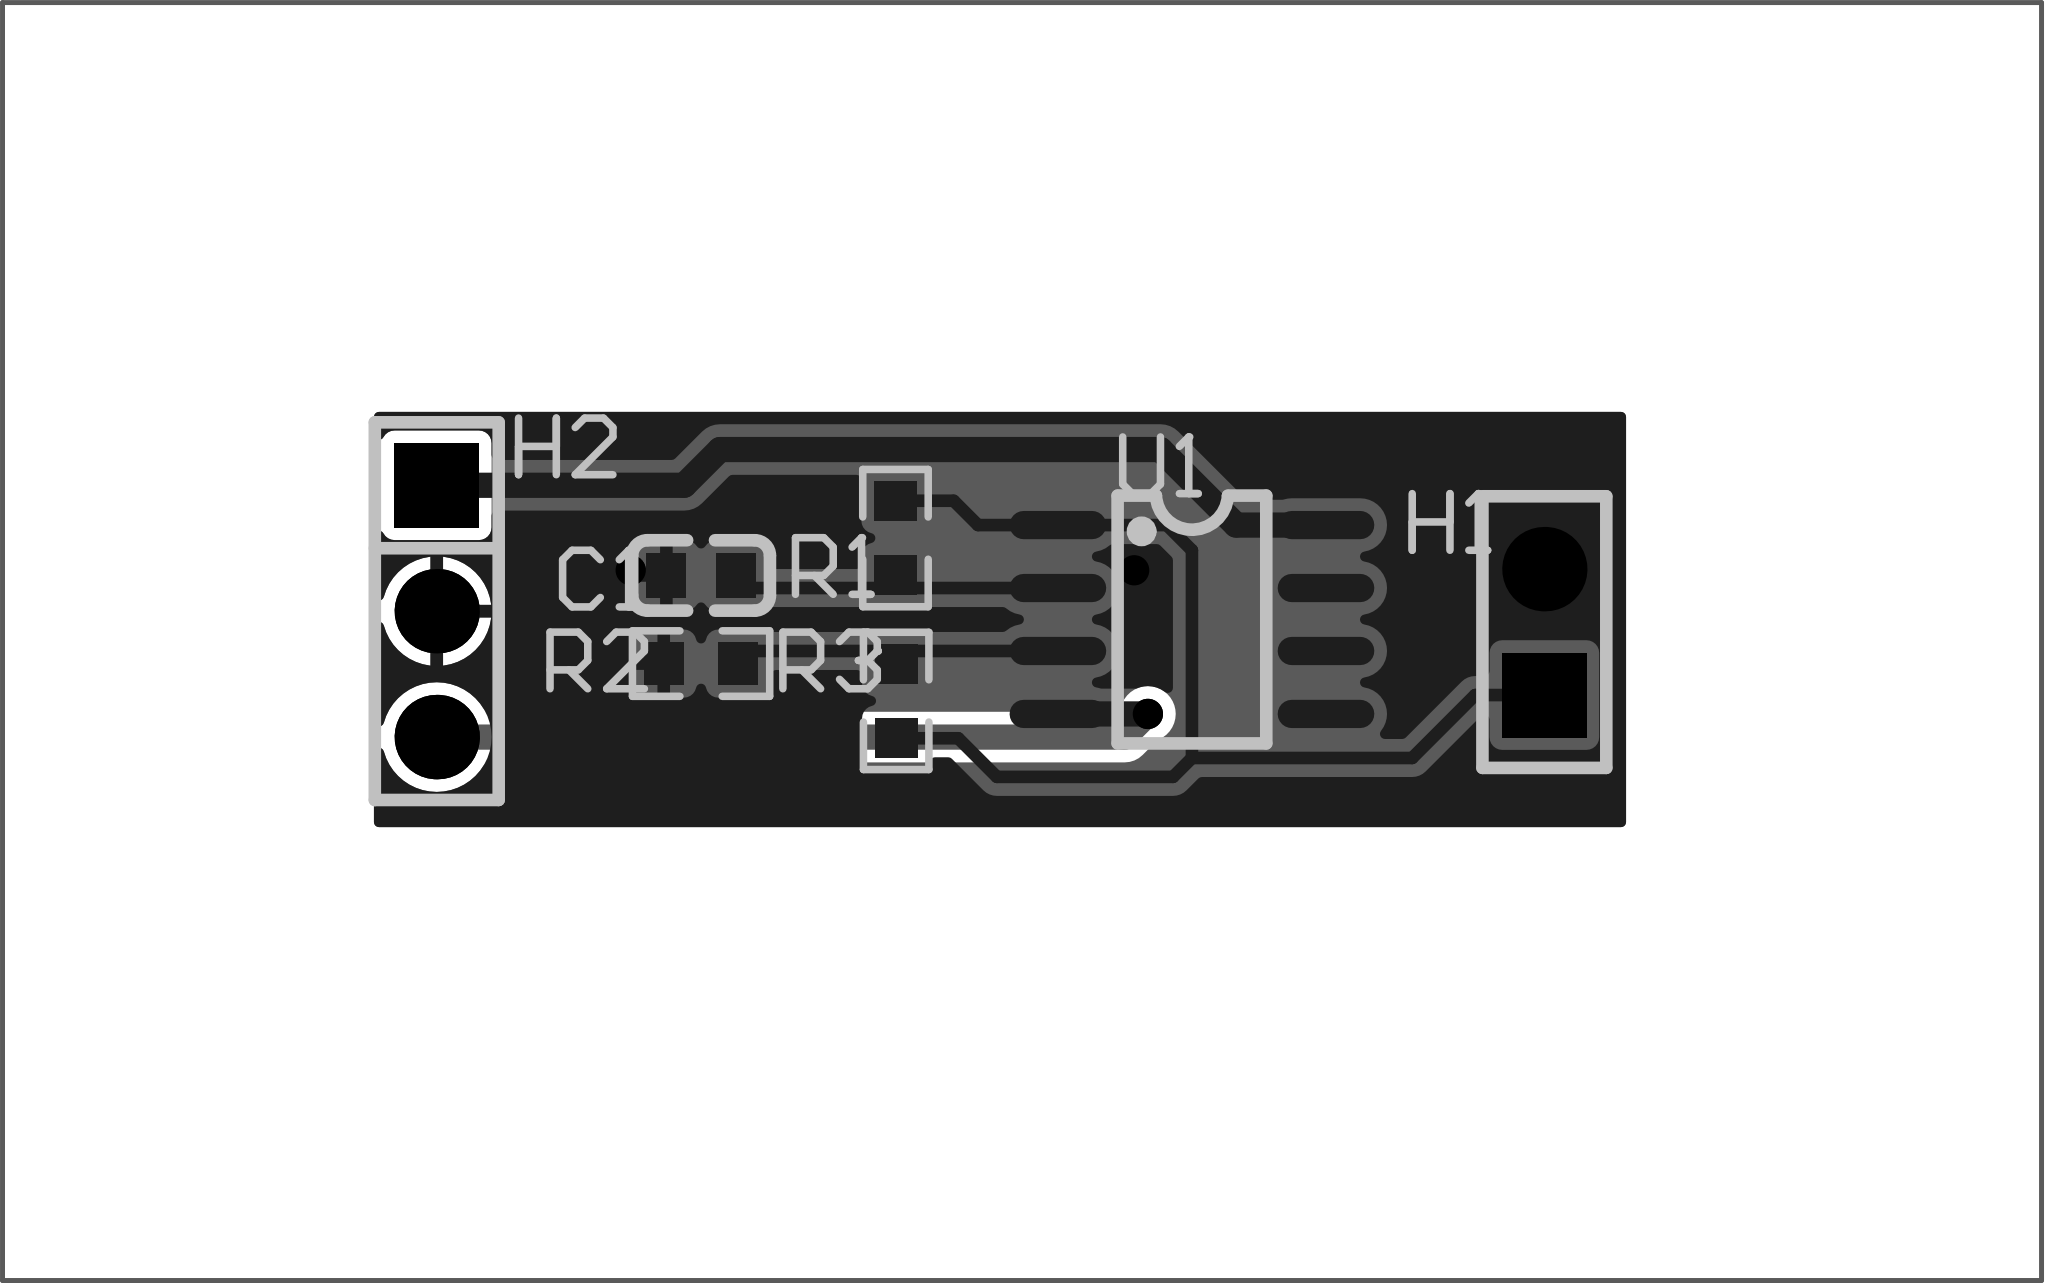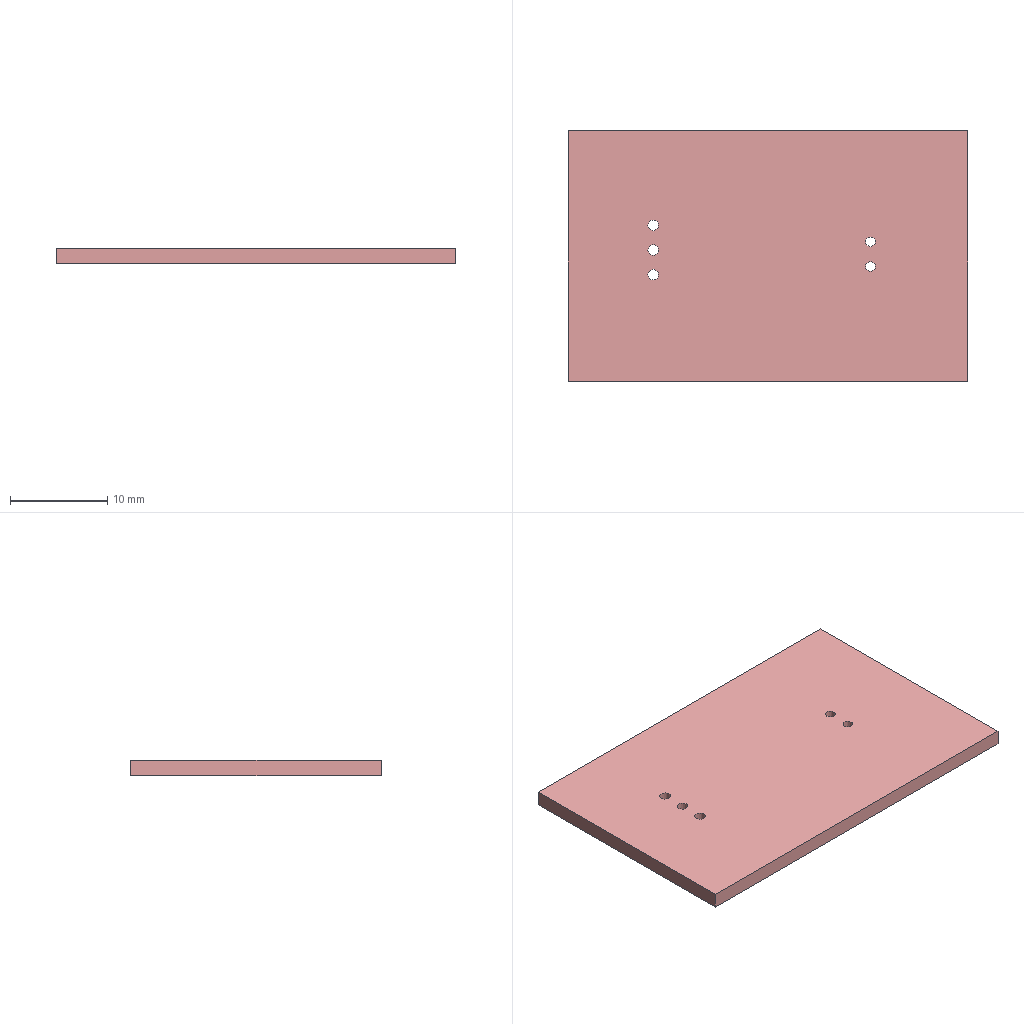Circuit board layout | Altium Designer | box 41.1 x 25.8 x 1.6 mm
Layer stack:
# Altium Designer layer stack of  (unit mm; dielectric type: 0 none, 1 core, 2 prepreg, 3 surface material)
index,name,kind,layer,copper_thickness_mm,dielectric_type,dielectric_thickness_mm,dielectric_material,dielectric_constant
0,Top Paste Mask Layer,other,,,,,,
1,Top Silkscreen Layer,other,,,,,,
2,Top Solder Mask Layer,dielectric,,,3,0.01,,3.3
3,Top Layer,copper,Top Layer,0.035,,,,
4,Dielectric1,dielectric,,,3,1.51,FR4,4.5
5,Bottom Layer,copper,Bottom Layer,0.035,,,,
6,Bottom Solder Mask Layer,dielectric,,,3,0.01,,3.3
7,Bottom Silkscreen Layer,other,,,,,,
8,Bottom Paste Mask Layer,other,,,,,,
# drill layer pairs: low layer,high layer
drill_pair,Top Layer,Bottom Layer
Part placement:
Designator,Comment,Layer,Footprint,Center-X(mm),Center-Y(mm),Rotation
C1,100nF,TopLayer,C0603,83.947,84.074,0
H1,,TopLayer,HDR-TH_2P-P2.54-V-F,100.965,82.931,90
H2,,TopLayer,HDR-TH_3P-P2.54-V-M,78.613,83.353,270
R1,10K,TopLayer,R0603,87.87,84.827,90
R2,10K,TopLayer,R0603,83.947,82.296,0
R3,10K,TopLayer,R0603,87.884,81.543,270
U1,NE5532DRG4,TopLayer,SOIC-8_L5.0-W4.0-P1.27-LS6.0-BL,93.853,83.185,270
Pad and via stacks:
# Altium Designer via and pad stacks of  (unit mm). Each distinct definition once, with the count of objects using it.
# via: kind,start_layer,end_layer,hole_mm,diameter_mm,mode(0 simple;1 top-mid-bottom;2 full stack),diameter_per_layer,count,example_net
# pad: kind,layer,hole_mm,hole_type(0 round;1 square;2 slot),plating,top_size,top_shape(1 round;2 rect;3 octagon;9 rounded rect),mid_size,bottom_size,mode,footprint,size_per_layer,count,example
pad,Top Layer,0,0,plated,0.8x0.9,2,0.8x0.9,0.8x0.9,0,C0603,,2,C1.2
pad,Top Layer,0,0,plated,0.8065x0.864,2,0.8065x0.864,0.8065x0.864,0,R0603,,6,R1.2
pad,Top Layer,0,0,plated,0.5684x1.95,1,0.5684x1.95,0.5684x1.95,0,SOIC-8_L5.0-W4.0-P1.27-LS6.0-BL,,8,U1.1
pad,Multi-Layer,1,0,plated,1.7x1.7,2,1.7x1.7,1.7x1.7,0,HDR-TH_2P-P2.54-V-F,,1,H1.1
pad,Multi-Layer,1,0,plated,1.7x1.7,1,1.7x1.7,1.7x1.7,0,HDR-TH_2P-P2.54-V-F,,1,H1.2
pad,Multi-Layer,1.1,0,plated,1.7x1.7,2,1.7x1.7,1.7x1.7,0,HDR-TH_3P-P2.54-V-M,,1,H2.1
pad,Multi-Layer,1.1,0,plated,1.7x1.7,1,1.7x1.7,1.7x1.7,0,HDR-TH_3P-P2.54-V-M,,2,H2.2
via,Top Layer,Bottom Layer,0.3048,0.61,0,,3,-VCC
Copper pours:
name,layer,net,type(0 solid;1 hatched;2 none)
Top Layer-GND,Top Layer,GND,0
Bottom Layer-GND,Bottom Layer,GND,0